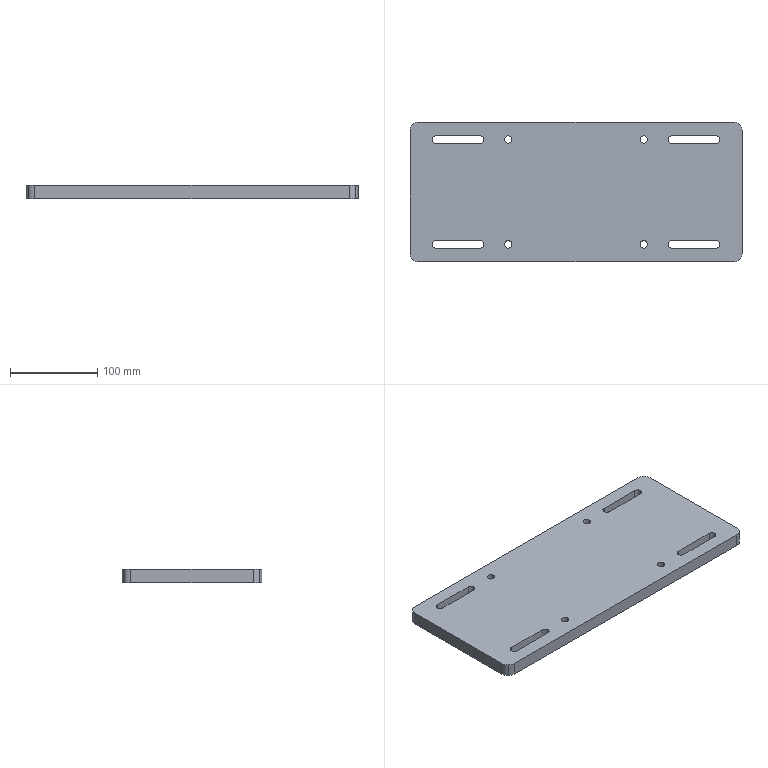Part | STEP file | DCV-000-005 | 1 solid | 38 faces | box 380 x 160 x 15 mm | volume 876589 mm3 | cylinder 24 | plane 14 | commonest cylinder face diameters 8.376 x8 9 x8 20 x8